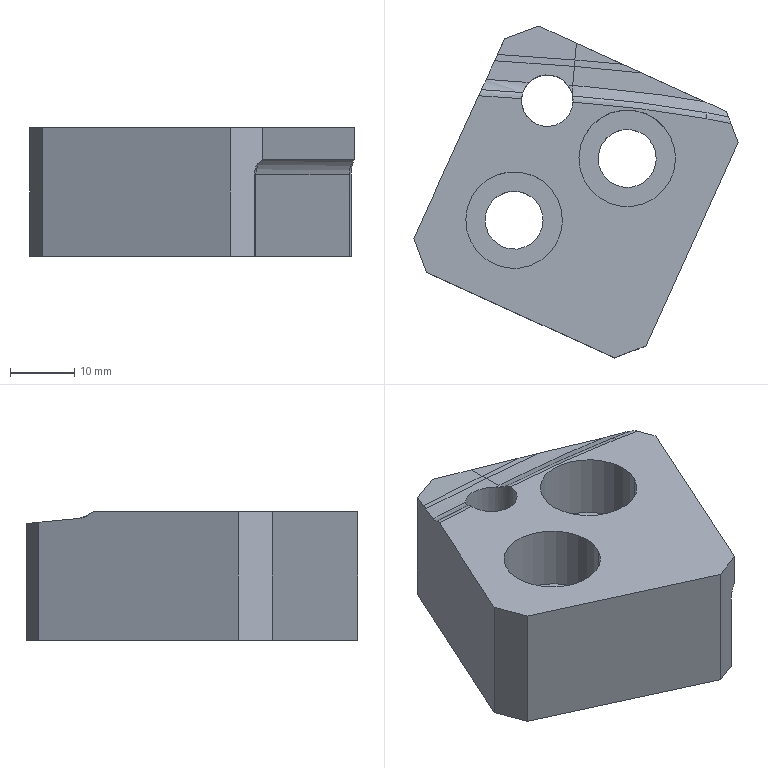Part | CATIA | 1 solid | 41 faces | box 50.331 x 51.489 x 20 mm | volume 26197 mm3 | plane 14 | spline 14 | cylinder 11 | other 2 | commonest cylinder face diameters 9 x4 15 x4 8 x2 6 x1